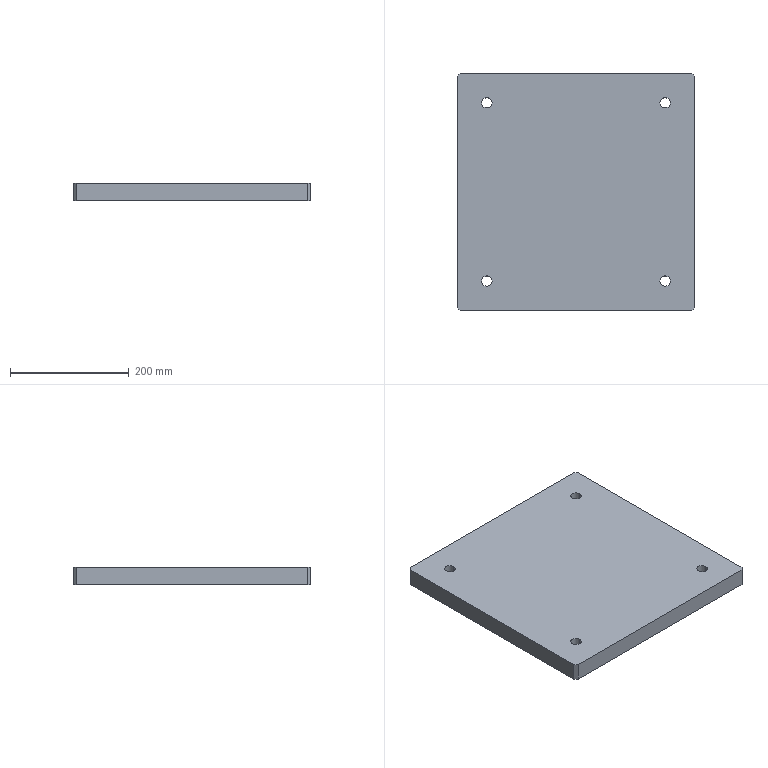Part | NX | features BREP 1 | 1 solid | 18 faces | box 400 x 400 x 30 mm | volume 4769637 mm3 | plane 10 | cylinder 8 | commonest cylinder face diameters 17.5 x8
STEP:
#1=CARTESIAN_POINT('',(-158.75,150.,0.));
#2=VERTEX_POINT('',#1);
#3=CARTESIAN_POINT('',(-141.25,150.,0.));
#4=VERTEX_POINT('',#3);
#5=CARTESIAN_POINT('',(-150.,150.,0.));
#6=DIRECTION('',(0.,0.,1.));
#7=DIRECTION('',(1.,0.,0.));
#8=AXIS2_PLACEMENT_3D('',#5,#6,#7);
#9=CIRCLE('',#8,8.75);
#10=EDGE_CURVE('',#2,#4,#9,.T.);
#11=ORIENTED_EDGE('',*,*,#10,.F.);
#12=CARTESIAN_POINT('',(-158.75,150.,30.));
#13=VERTEX_POINT('',#12);
#14=CARTESIAN_POINT('',(-158.75,150.,30.));
#15=DIRECTION('',(0.,0.,1.));
#16=VECTOR('',#15,1000.);
#17=LINE('',#14,#16);
#18=EDGE_CURVE('',#13,#2,#17,.F.);
#19=ORIENTED_EDGE('',*,*,#18,.F.);
#20=CARTESIAN_POINT('',(-141.25,150.,30.));
#21=VERTEX_POINT('',#20);
#22=CARTESIAN_POINT('',(-150.,150.,30.));
#23=DIRECTION('',(0.,0.,1.));
#24=DIRECTION('',(1.,0.,0.));
#25=AXIS2_PLACEMENT_3D('',#22,#23,#24);
#26=CIRCLE('',#25,8.75);
#27=EDGE_CURVE('',#13,#21,#26,.T.);
#28=ORIENTED_EDGE('',*,*,#27,.T.);
#29=CARTESIAN_POINT('',(-141.25,150.,30.));
#30=DIRECTION('',(0.,0.,1.));
#31=VECTOR('',#30,1000.);
#32=LINE('',#29,#31);
#33=EDGE_CURVE('',#21,#4,#32,.F.);
#34=ORIENTED_EDGE('',*,*,#33,.T.);
#35=EDGE_LOOP('',(#11,#19,#28,#34));
#36=FACE_BOUND('',#35,.T.);
#37=CARTESIAN_POINT('',(-150.,150.,30.));
#38=DIRECTION('',(0.,0.,1.));
#39=DIRECTION('',(1.,0.,0.));
#40=AXIS2_PLACEMENT_3D('',#37,#38,#39);
#41=CYLINDRICAL_SURFACE('',#40,8.75);
#42=ADVANCED_FACE('',(#36),#41,.F.);
#43=CARTESIAN_POINT('',(141.25,150.,0.));
#44=VERTEX_POINT('',#43);
#45=CARTESIAN_POINT('',(158.75,150.,0.));
#46=VERTEX_POINT('',#45);
#47=CARTESIAN_POINT('',(150.,150.,0.));
#48=DIRECTION('',(0.,0.,1.));
#49=DIRECTION('',(1.,0.,0.));
#50=AXIS2_PLACEMENT_3D('',#47,#48,#49);
#51=CIRCLE('',#50,8.75);
#52=EDGE_CURVE('',#44,#46,#51,.T.);
#53=ORIENTED_EDGE('',*,*,#52,.F.);
#54=CARTESIAN_POINT('',(141.25,150.,30.));
#55=VERTEX_POINT('',#54);
#56=CARTESIAN_POINT('',(141.25,150.,30.));
#57=DIRECTION('',(0.,0.,1.));
#58=VECTOR('',#57,1000.);
#59=LINE('',#56,#58);
#60=EDGE_CURVE('',#55,#44,#59,.F.);
#61=ORIENTED_EDGE('',*,*,#60,.F.);
#62=CARTESIAN_POINT('',(158.75,150.,30.));
#63=VERTEX_POINT('',#62);
#64=CARTESIAN_POINT('',(150.,150.,30.));
#65=DIRECTION('',(0.,0.,1.));
#66=DIRECTION('',(1.,0.,0.));
#67=AXIS2_PLACEMENT_3D('',#64,#65,#66);
#68=CIRCLE('',#67,8.75);
#69=EDGE_CURVE('',#55,#63,#68,.T.);
#70=ORIENTED_EDGE('',*,*,#69,.T.);
#71=CARTESIAN_POINT('',(158.75,150.,30.));
#72=DIRECTION('',(0.,0.,1.));
#73=VECTOR('',#72,1000.);
#74=LINE('',#71,#73);
#75=EDGE_CURVE('',#63,#46,#74,.F.);
#76=ORIENTED_EDGE('',*,*,#75,.T.);
#77=EDGE_LOOP('',(#53,#61,#70,#76));
#78=FACE_BOUND('',#77,.T.);
#79=CARTESIAN_POINT('',(150.,150.,30.));
#80=DIRECTION('',(0.,0.,1.));
#81=DIRECTION('',(1.,0.,0.));
#82=AXIS2_PLACEMENT_3D('',#79,#80,#81);
#83=CYLINDRICAL_SURFACE('',#82,8.75);
#84=ADVANCED_FACE('',(#78),#83,.F.);
#85=CARTESIAN_POINT('',(141.25,-150.,0.));
#86=VERTEX_POINT('',#85);
#87=CARTESIAN_POINT('',(158.75,-150.,0.));
#88=VERTEX_POINT('',#87);
#89=CARTESIAN_POINT('',(150.,-150.,0.));
#90=DIRECTION('',(0.,0.,1.));
#91=DIRECTION('',(1.,0.,0.));
#92=AXIS2_PLACEMENT_3D('',#89,#90,#91);
#93=CIRCLE('',#92,8.75);
#94=EDGE_CURVE('',#86,#88,#93,.T.);
#95=ORIENTED_EDGE('',*,*,#94,.F.);
#96=CARTESIAN_POINT('',(141.25,-150.,30.));
#97=VERTEX_POINT('',#96);
#98=CARTESIAN_POINT('',(141.25,-150.,30.));
#99=DIRECTION('',(0.,0.,1.));
#100=VECTOR('',#99,1000.);
#101=LINE('',#98,#100);
#102=EDGE_CURVE('',#97,#86,#101,.F.);
#103=ORIENTED_EDGE('',*,*,#102,.F.);
#104=CARTESIAN_POINT('',(158.75,-150.,30.));
#105=VERTEX_POINT('',#104);
#106=CARTESIAN_POINT('',(150.,-150.,30.));
#107=DIRECTION('',(0.,0.,1.));
#108=DIRECTION('',(1.,0.,0.));
#109=AXIS2_PLACEMENT_3D('',#106,#107,#108);
#110=CIRCLE('',#109,8.75);
#111=EDGE_CURVE('',#97,#105,#110,.T.);
#112=ORIENTED_EDGE('',*,*,#111,.T.);
#113=CARTESIAN_POINT('',(158.75,-150.,30.));
#114=DIRECTION('',(0.,0.,1.));
#115=VECTOR('',#114,1000.);
#116=LINE('',#113,#115);
#117=EDGE_CURVE('',#105,#88,#116,.F.);
#118=ORIENTED_EDGE('',*,*,#117,.T.);
#119=EDGE_LOOP('',(#95,#103,#112,#118));
#120=FACE_BOUND('',#119,.T.);
#121=CARTESIAN_POINT('',(150.,-150.,30.));
#122=DIRECTION('',(0.,0.,1.));
#123=DIRECTION('',(1.,0.,0.));
#124=AXIS2_PLACEMENT_3D('',#121,#122,#123);
#125=CYLINDRICAL_SURFACE('',#124,8.75);
#126=ADVANCED_FACE('',(#120),#125,.F.);
#127=CARTESIAN_POINT('',(-158.75,-150.,0.));
#128=VERTEX_POINT('',#127);
#129=CARTESIAN_POINT('',(-141.25,-150.,0.));
#130=VERTEX_POINT('',#129);
#131=CARTESIAN_POINT('',(-150.,-150.,0.));
#132=DIRECTION('',(0.,0.,1.));
#133=DIRECTION('',(1.,0.,0.));
#134=AXIS2_PLACEMENT_3D('',#131,#132,#133);
#135=CIRCLE('',#134,8.75);
#136=EDGE_CURVE('',#128,#130,#135,.T.);
#137=ORIENTED_EDGE('',*,*,#136,.F.);
#138=CARTESIAN_POINT('',(-158.75,-150.,30.));
#139=VERTEX_POINT('',#138);
#140=CARTESIAN_POINT('',(-158.75,-150.,30.));
#141=DIRECTION('',(0.,0.,1.));
#142=VECTOR('',#141,1000.);
#143=LINE('',#140,#142);
#144=EDGE_CURVE('',#139,#128,#143,.F.);
#145=ORIENTED_EDGE('',*,*,#144,.F.);
#146=CARTESIAN_POINT('',(-141.25,-150.,30.));
#147=VERTEX_POINT('',#146);
#148=CARTESIAN_POINT('',(-150.,-150.,30.));
#149=DIRECTION('',(0.,0.,1.));
#150=DIRECTION('',(1.,0.,0.));
#151=AXIS2_PLACEMENT_3D('',#148,#149,#150);
#152=CIRCLE('',#151,8.75);
#153=EDGE_CURVE('',#139,#147,#152,.T.);
#154=ORIENTED_EDGE('',*,*,#153,.T.);
#155=CARTESIAN_POINT('',(-141.25,-150.,30.));
#156=DIRECTION('',(0.,0.,1.));
#157=VECTOR('',#156,1000.);
#158=LINE('',#155,#157);
#159=EDGE_CURVE('',#147,#130,#158,.F.);
#160=ORIENTED_EDGE('',*,*,#159,.T.);
#161=EDGE_LOOP('',(#137,#145,#154,#160));
#162=FACE_BOUND('',#161,.T.);
#163=CARTESIAN_POINT('',(-150.,-150.,30.));
#164=DIRECTION('',(0.,0.,1.));
#165=DIRECTION('',(1.,0.,0.));
#166=AXIS2_PLACEMENT_3D('',#163,#164,#165);
#167=CYLINDRICAL_SURFACE('',#166,8.75);
#168=ADVANCED_FACE('',(#162),#167,.F.);
#169=CARTESIAN_POINT('',(200.,-195.,30.));
#170=VERTEX_POINT('',#169);
#171=CARTESIAN_POINT('',(200.,195.,30.));
#172=VERTEX_POINT('',#171);
#173=CARTESIAN_POINT('',(200.,200.,30.));
#174=DIRECTION('',(0.,1.,0.));
#175=VECTOR('',#174,1000.);
#176=LINE('',#173,#175);
#177=EDGE_CURVE('',#170,#172,#176,.T.);
#178=ORIENTED_EDGE('',*,*,#177,.F.);
#179=CARTESIAN_POINT('',(200.,-195.,0.));
#180=VERTEX_POINT('',#179);
#181=CARTESIAN_POINT('',(200.,-195.,30.));
#182=DIRECTION('',(0.,0.,-1.));
#183=VECTOR('',#182,1000.);
#184=LINE('',#181,#183);
#185=EDGE_CURVE('',#170,#180,#184,.T.);
#186=ORIENTED_EDGE('',*,*,#185,.T.);
#187=CARTESIAN_POINT('',(200.,195.,0.));
#188=VERTEX_POINT('',#187);
#189=CARTESIAN_POINT('',(200.,200.,0.));
#190=DIRECTION('',(0.,1.,0.));
#191=VECTOR('',#190,1000.);
#192=LINE('',#189,#191);
#193=EDGE_CURVE('',#180,#188,#192,.T.);
#194=ORIENTED_EDGE('',*,*,#193,.T.);
#195=CARTESIAN_POINT('',(200.,195.,30.));
#196=DIRECTION('',(0.,0.,1.));
#197=VECTOR('',#196,1000.);
#198=LINE('',#195,#197);
#199=EDGE_CURVE('',#188,#172,#198,.T.);
#200=ORIENTED_EDGE('',*,*,#199,.T.);
#201=EDGE_LOOP('',(#178,#186,#194,#200));
#202=FACE_BOUND('',#201,.T.);
#203=CARTESIAN_POINT('',(200.,200.,30.));
#204=DIRECTION('',(-1.,0.,0.));
#205=DIRECTION('',(0.,1.,0.));
#206=AXIS2_PLACEMENT_3D('',#203,#204,#205);
#207=PLANE('',#206);
#208=ADVANCED_FACE('',(#202),#207,.F.);
#209=CARTESIAN_POINT('',(195.,200.,30.));
#210=VERTEX_POINT('',#209);
#211=CARTESIAN_POINT('',(-195.,200.,30.));
#212=VERTEX_POINT('',#211);
#213=CARTESIAN_POINT('',(-200.,200.,30.));
#214=DIRECTION('',(-1.,0.,0.));
#215=VECTOR('',#214,1000.);
#216=LINE('',#213,#215);
#217=EDGE_CURVE('',#210,#212,#216,.T.);
#218=ORIENTED_EDGE('',*,*,#217,.F.);
#219=CARTESIAN_POINT('',(195.,200.,0.));
#220=VERTEX_POINT('',#219);
#221=CARTESIAN_POINT('',(195.,200.,30.));
#222=DIRECTION('',(0.,0.,-1.));
#223=VECTOR('',#222,1000.);
#224=LINE('',#221,#223);
#225=EDGE_CURVE('',#210,#220,#224,.T.);
#226=ORIENTED_EDGE('',*,*,#225,.T.);
#227=CARTESIAN_POINT('',(-195.,200.,0.));
#228=VERTEX_POINT('',#227);
#229=CARTESIAN_POINT('',(-200.,200.,0.));
#230=DIRECTION('',(-1.,0.,0.));
#231=VECTOR('',#230,1000.);
#232=LINE('',#229,#231);
#233=EDGE_CURVE('',#220,#228,#232,.T.);
#234=ORIENTED_EDGE('',*,*,#233,.T.);
#235=CARTESIAN_POINT('',(-195.,200.,30.));
#236=DIRECTION('',(0.,0.,1.));
#237=VECTOR('',#236,1000.);
#238=LINE('',#235,#237);
#239=EDGE_CURVE('',#228,#212,#238,.T.);
#240=ORIENTED_EDGE('',*,*,#239,.T.);
#241=EDGE_LOOP('',(#218,#226,#234,#240));
#242=FACE_BOUND('',#241,.T.);
#243=CARTESIAN_POINT('',(-200.,200.,30.));
#244=DIRECTION('',(0.,-1.,0.));
#245=DIRECTION('',(0.,0.,-1.));
#246=AXIS2_PLACEMENT_3D('',#243,#244,#245);
#247=PLANE('',#246);
#248=ADVANCED_FACE('',(#242),#247,.F.);
#249=CARTESIAN_POINT('',(-200.,195.,0.));
#250=VERTEX_POINT('',#249);
#251=CARTESIAN_POINT('',(-200.,-195.,0.));
#252=VERTEX_POINT('',#251);
#253=CARTESIAN_POINT('',(-200.,200.,0.));
#254=DIRECTION('',(0.,-1.,0.));
#255=VECTOR('',#254,1000.);
#256=LINE('',#253,#255);
#257=EDGE_CURVE('',#250,#252,#256,.T.);
#258=ORIENTED_EDGE('',*,*,#257,.T.);
#259=CARTESIAN_POINT('',(-200.,-195.,30.));
#260=VERTEX_POINT('',#259);
#261=CARTESIAN_POINT('',(-200.,-195.,30.));
#262=DIRECTION('',(0.,0.,1.));
#263=VECTOR('',#262,1000.);
#264=LINE('',#261,#263);
#265=EDGE_CURVE('',#252,#260,#264,.T.);
#266=ORIENTED_EDGE('',*,*,#265,.T.);
#267=CARTESIAN_POINT('',(-200.,195.,30.));
#268=VERTEX_POINT('',#267);
#269=CARTESIAN_POINT('',(-200.,200.,30.));
#270=DIRECTION('',(0.,-1.,0.));
#271=VECTOR('',#270,1000.);
#272=LINE('',#269,#271);
#273=EDGE_CURVE('',#268,#260,#272,.T.);
#274=ORIENTED_EDGE('',*,*,#273,.F.);
#275=CARTESIAN_POINT('',(-200.,195.,30.));
#276=DIRECTION('',(0.,0.,-1.));
#277=VECTOR('',#276,1000.);
#278=LINE('',#275,#277);
#279=EDGE_CURVE('',#268,#250,#278,.T.);
#280=ORIENTED_EDGE('',*,*,#279,.T.);
#281=EDGE_LOOP('',(#258,#266,#274,#280));
#282=FACE_BOUND('',#281,.T.);
#283=CARTESIAN_POINT('',(-200.,200.,30.));
#284=DIRECTION('',(1.,0.,0.));
#285=DIRECTION('',(0.,1.,0.));
#286=AXIS2_PLACEMENT_3D('',#283,#284,#285);
#287=PLANE('',#286);
#288=ADVANCED_FACE('',(#282),#287,.F.);
#289=CARTESIAN_POINT('',(-195.,-200.,30.));
#290=VERTEX_POINT('',#289);
#291=CARTESIAN_POINT('',(195.,-200.,30.));
#292=VERTEX_POINT('',#291);
#293=CARTESIAN_POINT('',(-200.,-200.,30.));
#294=DIRECTION('',(1.,0.,0.));
#295=VECTOR('',#294,1000.);
#296=LINE('',#293,#295);
#297=EDGE_CURVE('',#290,#292,#296,.T.);
#298=ORIENTED_EDGE('',*,*,#297,.F.);
#299=CARTESIAN_POINT('',(-195.,-200.,0.));
#300=VERTEX_POINT('',#299);
#301=CARTESIAN_POINT('',(-195.,-200.,30.));
#302=DIRECTION('',(0.,0.,-1.));
#303=VECTOR('',#302,1000.);
#304=LINE('',#301,#303);
#305=EDGE_CURVE('',#290,#300,#304,.T.);
#306=ORIENTED_EDGE('',*,*,#305,.T.);
#307=CARTESIAN_POINT('',(195.,-200.,0.));
#308=VERTEX_POINT('',#307);
#309=CARTESIAN_POINT('',(-200.,-200.,0.));
#310=DIRECTION('',(1.,0.,0.));
#311=VECTOR('',#310,1000.);
#312=LINE('',#309,#311);
#313=EDGE_CURVE('',#300,#308,#312,.T.);
#314=ORIENTED_EDGE('',*,*,#313,.T.);
#315=CARTESIAN_POINT('',(195.,-200.,30.));
#316=DIRECTION('',(0.,0.,1.));
#317=VECTOR('',#316,1000.);
#318=LINE('',#315,#317);
#319=EDGE_CURVE('',#308,#292,#318,.T.);
#320=ORIENTED_EDGE('',*,*,#319,.T.);
#321=EDGE_LOOP('',(#298,#306,#314,#320));
#322=FACE_BOUND('',#321,.T.);
#323=CARTESIAN_POINT('',(-200.,-200.,30.));
#324=DIRECTION('',(0.,1.,0.));
#325=DIRECTION('',(1.,0.,0.));
#326=AXIS2_PLACEMENT_3D('',#323,#324,#325);
#327=PLANE('',#326);
#328=ADVANCED_FACE('',(#322),#327,.F.);
#329=ORIENTED_EDGE('',*,*,#273,.T.);
#330=CARTESIAN_POINT('',(-197.5,-197.5,30.));
#331=DIRECTION('',(0.7071,-0.7071,0.));
#332=VECTOR('',#331,1000.);
#333=LINE('',#330,#332);
#334=EDGE_CURVE('',#260,#290,#333,.T.);
#335=ORIENTED_EDGE('',*,*,#334,.T.);
#336=ORIENTED_EDGE('',*,*,#297,.T.);
#337=CARTESIAN_POINT('',(197.5,-197.5,30.));
#338=DIRECTION('',(0.7071,0.7071,0.));
#339=VECTOR('',#338,1000.);
#340=LINE('',#337,#339);
#341=EDGE_CURVE('',#292,#170,#340,.T.);
#342=ORIENTED_EDGE('',*,*,#341,.T.);
#343=ORIENTED_EDGE('',*,*,#177,.T.);
#344=CARTESIAN_POINT('',(197.5,197.5,30.));
#345=DIRECTION('',(-0.7071,0.7071,0.));
#346=VECTOR('',#345,1000.);
#347=LINE('',#344,#346);
#348=EDGE_CURVE('',#172,#210,#347,.T.);
#349=ORIENTED_EDGE('',*,*,#348,.T.);
#350=ORIENTED_EDGE('',*,*,#217,.T.);
#351=CARTESIAN_POINT('',(-197.5,197.5,30.));
#352=DIRECTION('',(-0.7071,-0.7071,0.));
#353=VECTOR('',#352,1000.);
#354=LINE('',#351,#353);
#355=EDGE_CURVE('',#212,#268,#354,.T.);
#356=ORIENTED_EDGE('',*,*,#355,.T.);
#357=EDGE_LOOP('',(#329,#335,#336,#342,#343,#349,#350,#356));
#358=FACE_BOUND('',#357,.T.);
#359=CARTESIAN_POINT('',(-150.,150.,30.));
#360=DIRECTION('',(0.,0.,1.));
#361=DIRECTION('',(1.,0.,0.));
#362=AXIS2_PLACEMENT_3D('',#359,#360,#361);
#363=CIRCLE('',#362,8.75);
#364=EDGE_CURVE('',#21,#13,#363,.T.);
#365=ORIENTED_EDGE('',*,*,#364,.F.);
#366=ORIENTED_EDGE('',*,*,#27,.F.);
#367=EDGE_LOOP('',(#365,#366));
#368=FACE_BOUND('',#367,.T.);
#369=CARTESIAN_POINT('',(150.,150.,30.));
#370=DIRECTION('',(0.,0.,1.));
#371=DIRECTION('',(1.,0.,0.));
#372=AXIS2_PLACEMENT_3D('',#369,#370,#371);
#373=CIRCLE('',#372,8.75);
#374=EDGE_CURVE('',#63,#55,#373,.T.);
#375=ORIENTED_EDGE('',*,*,#374,.F.);
#376=ORIENTED_EDGE('',*,*,#69,.F.);
#377=EDGE_LOOP('',(#375,#376));
#378=FACE_BOUND('',#377,.T.);
#379=CARTESIAN_POINT('',(150.,-150.,30.));
#380=DIRECTION('',(0.,0.,1.));
#381=DIRECTION('',(1.,0.,0.));
#382=AXIS2_PLACEMENT_3D('',#379,#380,#381);
#383=CIRCLE('',#382,8.75);
#384=EDGE_CURVE('',#105,#97,#383,.T.);
#385=ORIENTED_EDGE('',*,*,#384,.F.);
#386=ORIENTED_EDGE('',*,*,#111,.F.);
#387=EDGE_LOOP('',(#385,#386));
#388=FACE_BOUND('',#387,.T.);
#389=CARTESIAN_POINT('',(-150.,-150.,30.));
#390=DIRECTION('',(0.,0.,1.));
#391=DIRECTION('',(1.,0.,0.));
#392=AXIS2_PLACEMENT_3D('',#389,#390,#391);
#393=CIRCLE('',#392,8.75);
#394=EDGE_CURVE('',#147,#139,#393,.T.);
#395=ORIENTED_EDGE('',*,*,#394,.F.);
#396=ORIENTED_EDGE('',*,*,#153,.F.);
#397=EDGE_LOOP('',(#395,#396));
#398=FACE_BOUND('',#397,.T.);
#399=CARTESIAN_POINT('',(0.,0.,30.));
#400=DIRECTION('',(0.,0.,1.));
#401=DIRECTION('',(1.,0.,0.));
#402=AXIS2_PLACEMENT_3D('',#399,#400,#401);
#403=PLANE('',#402);
#404=ADVANCED_FACE('',(#358,#368,#378,#388,#398),#403,.T.);
#405=ORIENTED_EDGE('',*,*,#313,.F.);
#406=CARTESIAN_POINT('',(-195.,-200.,0.));
#407=DIRECTION('',(-0.7071,0.7071,0.));
#408=VECTOR('',#407,1000.);
#409=LINE('',#406,#408);
#410=EDGE_CURVE('',#300,#252,#409,.T.);
#411=ORIENTED_EDGE('',*,*,#410,.T.);
#412=ORIENTED_EDGE('',*,*,#257,.F.);
#413=CARTESIAN_POINT('',(-200.,195.,0.));
#414=DIRECTION('',(0.7071,0.7071,0.));
#415=VECTOR('',#414,1000.);
#416=LINE('',#413,#415);
#417=EDGE_CURVE('',#250,#228,#416,.T.);
#418=ORIENTED_EDGE('',*,*,#417,.T.);
#419=ORIENTED_EDGE('',*,*,#233,.F.);
#420=CARTESIAN_POINT('',(195.,200.,0.));
#421=DIRECTION('',(0.7071,-0.7071,0.));
#422=VECTOR('',#421,1000.);
#423=LINE('',#420,#422);
#424=EDGE_CURVE('',#220,#188,#423,.T.);
#425=ORIENTED_EDGE('',*,*,#424,.T.);
#426=ORIENTED_EDGE('',*,*,#193,.F.);
#427=CARTESIAN_POINT('',(200.,-195.,0.));
#428=DIRECTION('',(-0.7071,-0.7071,0.));
#429=VECTOR('',#428,1000.);
#430=LINE('',#427,#429);
#431=EDGE_CURVE('',#180,#308,#430,.T.);
#432=ORIENTED_EDGE('',*,*,#431,.T.);
#433=EDGE_LOOP('',(#405,#411,#412,#418,#419,#425,#426,#432));
#434=FACE_BOUND('',#433,.T.);
#435=CARTESIAN_POINT('',(-150.,150.,0.));
#436=DIRECTION('',(0.,0.,1.));
#437=DIRECTION('',(1.,0.,0.));
#438=AXIS2_PLACEMENT_3D('',#435,#436,#437);
#439=CIRCLE('',#438,8.75);
#440=EDGE_CURVE('',#4,#2,#439,.T.);
#441=ORIENTED_EDGE('',*,*,#440,.T.);
#442=ORIENTED_EDGE('',*,*,#10,.T.);
#443=EDGE_LOOP('',(#441,#442));
#444=FACE_BOUND('',#443,.T.);
#445=CARTESIAN_POINT('',(150.,150.,0.));
#446=DIRECTION('',(0.,0.,1.));
#447=DIRECTION('',(1.,0.,0.));
#448=AXIS2_PLACEMENT_3D('',#445,#446,#447);
#449=CIRCLE('',#448,8.75);
#450=EDGE_CURVE('',#46,#44,#449,.T.);
#451=ORIENTED_EDGE('',*,*,#450,.T.);
#452=ORIENTED_EDGE('',*,*,#52,.T.);
#453=EDGE_LOOP('',(#451,#452));
#454=FACE_BOUND('',#453,.T.);
#455=CARTESIAN_POINT('',(150.,-150.,0.));
#456=DIRECTION('',(0.,0.,1.));
#457=DIRECTION('',(1.,0.,0.));
#458=AXIS2_PLACEMENT_3D('',#455,#456,#457);
#459=CIRCLE('',#458,8.75);
#460=EDGE_CURVE('',#88,#86,#459,.T.);
#461=ORIENTED_EDGE('',*,*,#460,.T.);
#462=ORIENTED_EDGE('',*,*,#94,.T.);
#463=EDGE_LOOP('',(#461,#462));
#464=FACE_BOUND('',#463,.T.);
#465=CARTESIAN_POINT('',(-150.,-150.,0.));
#466=DIRECTION('',(0.,0.,1.));
#467=DIRECTION('',(1.,0.,0.));
#468=AXIS2_PLACEMENT_3D('',#465,#466,#467);
#469=CIRCLE('',#468,8.75);
#470=EDGE_CURVE('',#130,#128,#469,.T.);
#471=ORIENTED_EDGE('',*,*,#470,.T.);
#472=ORIENTED_EDGE('',*,*,#136,.T.);
#473=EDGE_LOOP('',(#471,#472));
#474=FACE_BOUND('',#473,.T.);
#475=CARTESIAN_POINT('',(0.,0.,0.));
#476=DIRECTION('',(0.,0.,1.));
#477=DIRECTION('',(1.,0.,0.));
#478=AXIS2_PLACEMENT_3D('',#475,#476,#477);
#479=PLANE('',#478);
#480=ADVANCED_FACE('',(#434,#444,#454,#464,#474),#479,.F.);
#481=ORIENTED_EDGE('',*,*,#334,.F.);
#482=ORIENTED_EDGE('',*,*,#265,.F.);
#483=ORIENTED_EDGE('',*,*,#410,.F.);
#484=ORIENTED_EDGE('',*,*,#305,.F.);
#485=EDGE_LOOP('',(#481,#482,#483,#484));
#486=FACE_BOUND('',#485,.T.);
#487=CARTESIAN_POINT('',(-195.,-200.,30.));
#488=DIRECTION('',(0.7071,0.7071,0.));
#489=DIRECTION('',(0.,0.,-1.));
#490=AXIS2_PLACEMENT_3D('',#487,#488,#489);
#491=PLANE('',#490);
#492=ADVANCED_FACE('',(#486),#491,.F.);
#493=ORIENTED_EDGE('',*,*,#341,.F.);
#494=ORIENTED_EDGE('',*,*,#319,.F.);
#495=ORIENTED_EDGE('',*,*,#431,.F.);
#496=ORIENTED_EDGE('',*,*,#185,.F.);
#497=EDGE_LOOP('',(#493,#494,#495,#496));
#498=FACE_BOUND('',#497,.T.);
#499=CARTESIAN_POINT('',(200.,-195.,30.));
#500=DIRECTION('',(-0.7071,0.7071,0.));
#501=DIRECTION('',(0.,0.,1.));
#502=AXIS2_PLACEMENT_3D('',#499,#500,#501);
#503=PLANE('',#502);
#504=ADVANCED_FACE('',(#498),#503,.F.);
#505=ORIENTED_EDGE('',*,*,#348,.F.);
#506=ORIENTED_EDGE('',*,*,#199,.F.);
#507=ORIENTED_EDGE('',*,*,#424,.F.);
#508=ORIENTED_EDGE('',*,*,#225,.F.);
#509=EDGE_LOOP('',(#505,#506,#507,#508));
#510=FACE_BOUND('',#509,.T.);
#511=CARTESIAN_POINT('',(195.,200.,30.));
#512=DIRECTION('',(-0.7071,-0.7071,0.));
#513=DIRECTION('',(-0.7071,0.7071,0.));
#514=AXIS2_PLACEMENT_3D('',#511,#512,#513);
#515=PLANE('',#514);
#516=ADVANCED_FACE('',(#510),#515,.F.);
#517=ORIENTED_EDGE('',*,*,#355,.F.);
#518=ORIENTED_EDGE('',*,*,#239,.F.);
#519=ORIENTED_EDGE('',*,*,#417,.F.);
#520=ORIENTED_EDGE('',*,*,#279,.F.);
#521=EDGE_LOOP('',(#517,#518,#519,#520));
#522=FACE_BOUND('',#521,.T.);
#523=CARTESIAN_POINT('',(-200.,195.,30.));
#524=DIRECTION('',(0.7071,-0.7071,0.));
#525=DIRECTION('',(0.,0.,-1.));
#526=AXIS2_PLACEMENT_3D('',#523,#524,#525);
#527=PLANE('',#526);
#528=ADVANCED_FACE('',(#522),#527,.F.);
#529=ORIENTED_EDGE('',*,*,#144,.T.);
#530=ORIENTED_EDGE('',*,*,#470,.F.);
#531=ORIENTED_EDGE('',*,*,#159,.F.);
#532=ORIENTED_EDGE('',*,*,#394,.T.);
#533=EDGE_LOOP('',(#529,#530,#531,#532));
#534=FACE_BOUND('',#533,.T.);
#535=CARTESIAN_POINT('',(-150.,-150.,30.));
#536=DIRECTION('',(0.,0.,1.));
#537=DIRECTION('',(1.,0.,0.));
#538=AXIS2_PLACEMENT_3D('',#535,#536,#537);
#539=CYLINDRICAL_SURFACE('',#538,8.75);
#540=ADVANCED_FACE('',(#534),#539,.F.);
#541=ORIENTED_EDGE('',*,*,#102,.T.);
#542=ORIENTED_EDGE('',*,*,#460,.F.);
#543=ORIENTED_EDGE('',*,*,#117,.F.);
#544=ORIENTED_EDGE('',*,*,#384,.T.);
#545=EDGE_LOOP('',(#541,#542,#543,#544));
#546=FACE_BOUND('',#545,.T.);
#547=CARTESIAN_POINT('',(150.,-150.,30.));
#548=DIRECTION('',(0.,0.,1.));
#549=DIRECTION('',(1.,0.,0.));
#550=AXIS2_PLACEMENT_3D('',#547,#548,#549);
#551=CYLINDRICAL_SURFACE('',#550,8.75);
#552=ADVANCED_FACE('',(#546),#551,.F.);
#553=ORIENTED_EDGE('',*,*,#60,.T.);
#554=ORIENTED_EDGE('',*,*,#450,.F.);
#555=ORIENTED_EDGE('',*,*,#75,.F.);
#556=ORIENTED_EDGE('',*,*,#374,.T.);
#557=EDGE_LOOP('',(#553,#554,#555,#556));
#558=FACE_BOUND('',#557,.T.);
#559=CARTESIAN_POINT('',(150.,150.,30.));
#560=DIRECTION('',(0.,0.,1.));
#561=DIRECTION('',(1.,0.,0.));
#562=AXIS2_PLACEMENT_3D('',#559,#560,#561);
#563=CYLINDRICAL_SURFACE('',#562,8.75);
#564=ADVANCED_FACE('',(#558),#563,.F.);
#565=ORIENTED_EDGE('',*,*,#18,.T.);
#566=ORIENTED_EDGE('',*,*,#440,.F.);
#567=ORIENTED_EDGE('',*,*,#33,.F.);
#568=ORIENTED_EDGE('',*,*,#364,.T.);
#569=EDGE_LOOP('',(#565,#566,#567,#568));
#570=FACE_BOUND('',#569,.T.);
#571=CARTESIAN_POINT('',(-150.,150.,30.));
#572=DIRECTION('',(0.,0.,1.));
#573=DIRECTION('',(1.,0.,0.));
#574=AXIS2_PLACEMENT_3D('',#571,#572,#573);
#575=CYLINDRICAL_SURFACE('',#574,8.75);
#576=ADVANCED_FACE('',(#570),#575,.F.);
#577=CLOSED_SHELL('',(#42,#84,#126,#168,#208,#248,#288,#328,#404,#480,#492,#504,#516,#528,#540,#552,#564,#576));
#578=MANIFOLD_SOLID_BREP('',#577);
#579=(LENGTH_UNIT()NAMED_UNIT(*)SI_UNIT(.MILLI.,.METRE.));
#580=UNCERTAINTY_MEASURE_WITH_UNIT(LENGTH_MEASURE(0.00001),#579,'','');
#581=(NAMED_UNIT(*)PLANE_ANGLE_UNIT()SI_UNIT($,.RADIAN.));
#582=(NAMED_UNIT(*)SI_UNIT($,.STERADIAN.)SOLID_ANGLE_UNIT());
#583=(GEOMETRIC_REPRESENTATION_CONTEXT(3)GLOBAL_UNCERTAINTY_ASSIGNED_CONTEXT((#580))GLOBAL_UNIT_ASSIGNED_CONTEXT((#579,#581,#582))REPRESENTATION_CONTEXT('',''));
#584=ADVANCED_BREP_SHAPE_REPRESENTATION('',(#578),#583);